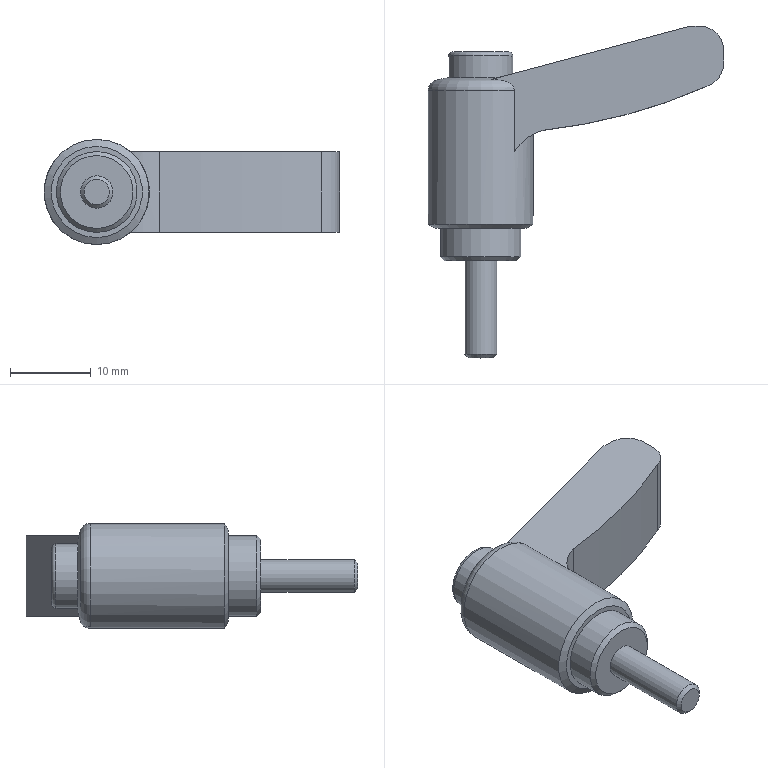Part | STEP file | CLDMC4-12-M | 2 solids | 40 faces | box 36.5 x 41 x 13 mm | volume 4938 mm3 | plane 23 | cylinder 10 | cone 4 | torus 2 | sphere 1 | commonest cylinder face diameters 6 x2 8 x2 10 x2 4 x1 12 x1 13 x1
STEP:
#1=CARTESIAN_POINT('',(-1.5,23.8,0.866));
#2=VERTEX_POINT('',#1);
#3=CARTESIAN_POINT('',(-0.75,23.8,1.299));
#4=VERTEX_POINT('',#3);
#5=CARTESIAN_POINT('',(-1.5,23.8,0.866));
#6=DIRECTION('',(0.866,0.,0.5));
#7=VECTOR('',#6,1000.);
#8=LINE('',#5,#7);
#9=EDGE_CURVE('',#2,#4,#8,.T.);
#10=ORIENTED_EDGE('',*,*,#9,.T.);
#11=CARTESIAN_POINT('',(-1.5,23.8,0.));
#12=VERTEX_POINT('',#11);
#13=CARTESIAN_POINT('',(0.,23.8,0.));
#14=DIRECTION('',(0.,1.,0.));
#15=DIRECTION('',(0.,0.,1.));
#16=AXIS2_PLACEMENT_3D('',#13,#14,#15);
#17=CIRCLE('',#16,1.5);
#18=EDGE_CURVE('',#4,#12,#17,.F.);
#19=ORIENTED_EDGE('',*,*,#18,.T.);
#20=CARTESIAN_POINT('',(-1.5,23.8,-0.866));
#21=DIRECTION('',(0.,0.,1.));
#22=VECTOR('',#21,1000.);
#23=LINE('',#20,#22);
#24=EDGE_CURVE('',#12,#2,#23,.T.);
#25=ORIENTED_EDGE('',*,*,#24,.T.);
#26=EDGE_LOOP('',(#10,#19,#25));
#27=FACE_OUTER_BOUND('',#26,.T.);
#28=CARTESIAN_POINT('',(0.,23.8,0.));
#29=DIRECTION('',(0.,1.,0.));
#30=DIRECTION('',(0.,0.,1.));
#31=AXIS2_PLACEMENT_3D('',#28,#29,#30);
#32=PLANE('',#31);
#33=ADVANCED_FACE('',(#27),#32,.T.);
#34=CARTESIAN_POINT('',(-1.5,23.8,-0.866));
#35=VERTEX_POINT('',#34);
#36=CARTESIAN_POINT('',(-1.5,23.8,-0.866));
#37=DIRECTION('',(0.,0.,1.));
#38=VECTOR('',#37,1000.);
#39=LINE('',#36,#38);
#40=EDGE_CURVE('',#35,#12,#39,.T.);
#41=ORIENTED_EDGE('',*,*,#40,.T.);
#42=CARTESIAN_POINT('',(-0.75,23.8,-1.299));
#43=VERTEX_POINT('',#42);
#44=CARTESIAN_POINT('',(0.,23.8,0.));
#45=DIRECTION('',(0.,1.,0.));
#46=DIRECTION('',(0.,0.,1.));
#47=AXIS2_PLACEMENT_3D('',#44,#45,#46);
#48=CIRCLE('',#47,1.5);
#49=EDGE_CURVE('',#12,#43,#48,.F.);
#50=ORIENTED_EDGE('',*,*,#49,.T.);
#51=CARTESIAN_POINT('',(0.,23.8,-1.732));
#52=DIRECTION('',(-0.866,0.,0.5));
#53=VECTOR('',#52,1000.);
#54=LINE('',#51,#53);
#55=EDGE_CURVE('',#43,#35,#54,.T.);
#56=ORIENTED_EDGE('',*,*,#55,.T.);
#57=EDGE_LOOP('',(#41,#50,#56));
#58=FACE_OUTER_BOUND('',#57,.T.);
#59=CARTESIAN_POINT('',(0.,23.8,0.));
#60=DIRECTION('',(0.,1.,0.));
#61=DIRECTION('',(0.,0.,1.));
#62=AXIS2_PLACEMENT_3D('',#59,#60,#61);
#63=PLANE('',#62);
#64=ADVANCED_FACE('',(#58),#63,.T.);
#65=CARTESIAN_POINT('',(0.,23.8,-1.732));
#66=VERTEX_POINT('',#65);
#67=CARTESIAN_POINT('',(0.,23.8,-1.732));
#68=DIRECTION('',(-0.866,0.,0.5));
#69=VECTOR('',#68,1000.);
#70=LINE('',#67,#69);
#71=EDGE_CURVE('',#66,#43,#70,.T.);
#72=ORIENTED_EDGE('',*,*,#71,.T.);
#73=CARTESIAN_POINT('',(0.,23.8,-1.5));
#74=VERTEX_POINT('',#73);
#75=CARTESIAN_POINT('',(0.,23.8,0.));
#76=DIRECTION('',(0.,1.,0.));
#77=DIRECTION('',(0.,0.,1.));
#78=AXIS2_PLACEMENT_3D('',#75,#76,#77);
#79=CIRCLE('',#78,1.5);
#80=EDGE_CURVE('',#43,#74,#79,.F.);
#81=ORIENTED_EDGE('',*,*,#80,.T.);
#82=CARTESIAN_POINT('',(0.75,23.8,-1.299));
#83=VERTEX_POINT('',#82);
#84=CARTESIAN_POINT('',(0.,23.8,0.));
#85=DIRECTION('',(0.,1.,0.));
#86=DIRECTION('',(0.,0.,1.));
#87=AXIS2_PLACEMENT_3D('',#84,#85,#86);
#88=CIRCLE('',#87,1.5);
#89=EDGE_CURVE('',#74,#83,#88,.F.);
#90=ORIENTED_EDGE('',*,*,#89,.T.);
#91=CARTESIAN_POINT('',(1.5,23.8,-0.866));
#92=DIRECTION('',(-0.866,0.,-0.5));
#93=VECTOR('',#92,1000.);
#94=LINE('',#91,#93);
#95=EDGE_CURVE('',#83,#66,#94,.T.);
#96=ORIENTED_EDGE('',*,*,#95,.T.);
#97=EDGE_LOOP('',(#72,#81,#90,#96));
#98=FACE_OUTER_BOUND('',#97,.T.);
#99=CARTESIAN_POINT('',(0.,23.8,0.));
#100=DIRECTION('',(0.,1.,0.));
#101=DIRECTION('',(0.,0.,1.));
#102=AXIS2_PLACEMENT_3D('',#99,#100,#101);
#103=PLANE('',#102);
#104=ADVANCED_FACE('',(#98),#103,.T.);
#105=CARTESIAN_POINT('',(1.5,23.8,-0.866));
#106=VERTEX_POINT('',#105);
#107=CARTESIAN_POINT('',(1.5,23.8,-0.866));
#108=DIRECTION('',(-0.866,0.,-0.5));
#109=VECTOR('',#108,1000.);
#110=LINE('',#107,#109);
#111=EDGE_CURVE('',#106,#83,#110,.T.);
#112=ORIENTED_EDGE('',*,*,#111,.T.);
#113=CARTESIAN_POINT('',(1.5,23.8,0.));
#114=VERTEX_POINT('',#113);
#115=CARTESIAN_POINT('',(0.,23.8,0.));
#116=DIRECTION('',(0.,1.,0.));
#117=DIRECTION('',(0.,0.,1.));
#118=AXIS2_PLACEMENT_3D('',#115,#116,#117);
#119=CIRCLE('',#118,1.5);
#120=EDGE_CURVE('',#83,#114,#119,.F.);
#121=ORIENTED_EDGE('',*,*,#120,.T.);
#122=CARTESIAN_POINT('',(1.5,23.8,0.866));
#123=DIRECTION('',(0.,0.,-1.));
#124=VECTOR('',#123,1000.);
#125=LINE('',#122,#124);
#126=EDGE_CURVE('',#114,#106,#125,.T.);
#127=ORIENTED_EDGE('',*,*,#126,.T.);
#128=EDGE_LOOP('',(#112,#121,#127));
#129=FACE_OUTER_BOUND('',#128,.T.);
#130=CARTESIAN_POINT('',(0.,23.8,0.));
#131=DIRECTION('',(0.,1.,0.));
#132=DIRECTION('',(0.,0.,1.));
#133=AXIS2_PLACEMENT_3D('',#130,#131,#132);
#134=PLANE('',#133);
#135=ADVANCED_FACE('',(#129),#134,.T.);
#136=CARTESIAN_POINT('',(1.5,23.8,0.866));
#137=VERTEX_POINT('',#136);
#138=CARTESIAN_POINT('',(1.5,23.8,0.866));
#139=DIRECTION('',(0.,0.,-1.));
#140=VECTOR('',#139,1000.);
#141=LINE('',#138,#140);
#142=EDGE_CURVE('',#137,#114,#141,.T.);
#143=ORIENTED_EDGE('',*,*,#142,.T.);
#144=CARTESIAN_POINT('',(0.75,23.8,1.299));
#145=VERTEX_POINT('',#144);
#146=CARTESIAN_POINT('',(0.,23.8,0.));
#147=DIRECTION('',(0.,-1.,0.));
#148=DIRECTION('',(0.,0.,-1.));
#149=AXIS2_PLACEMENT_3D('',#146,#147,#148);
#150=CIRCLE('',#149,1.5);
#151=EDGE_CURVE('',#114,#145,#150,.T.);
#152=ORIENTED_EDGE('',*,*,#151,.T.);
#153=CARTESIAN_POINT('',(0.,23.8,1.732));
#154=DIRECTION('',(0.866,0.,-0.5));
#155=VECTOR('',#154,1000.);
#156=LINE('',#153,#155);
#157=EDGE_CURVE('',#145,#137,#156,.T.);
#158=ORIENTED_EDGE('',*,*,#157,.T.);
#159=EDGE_LOOP('',(#143,#152,#158));
#160=FACE_OUTER_BOUND('',#159,.T.);
#161=CARTESIAN_POINT('',(0.,23.8,0.));
#162=DIRECTION('',(0.,1.,0.));
#163=DIRECTION('',(0.,0.,1.));
#164=AXIS2_PLACEMENT_3D('',#161,#162,#163);
#165=PLANE('',#164);
#166=ADVANCED_FACE('',(#160),#165,.T.);
#167=CARTESIAN_POINT('',(0.,25.8,-3.5));
#168=VERTEX_POINT('',#167);
#169=CARTESIAN_POINT('',(0.,25.8,3.5));
#170=VERTEX_POINT('',#169);
#171=CARTESIAN_POINT('',(0.,25.8,0.));
#172=DIRECTION('',(0.,-1.,0.));
#173=DIRECTION('',(0.,0.,-1.));
#174=AXIS2_PLACEMENT_3D('',#171,#172,#173);
#175=CIRCLE('',#174,3.5);
#176=EDGE_CURVE('',#168,#170,#175,.T.);
#177=ORIENTED_EDGE('',*,*,#176,.F.);
#178=CARTESIAN_POINT('',(0.,25.8,0.));
#179=DIRECTION('',(0.,-1.,0.));
#180=DIRECTION('',(0.,0.,-1.));
#181=AXIS2_PLACEMENT_3D('',#178,#179,#180);
#182=CIRCLE('',#181,3.5);
#183=EDGE_CURVE('',#170,#168,#182,.T.);
#184=ORIENTED_EDGE('',*,*,#183,.F.);
#185=EDGE_LOOP('',(#177,#184));
#186=FACE_OUTER_BOUND('',#185,.T.);
#187=CARTESIAN_POINT('',(-1.5,25.8,-0.866));
#188=VERTEX_POINT('',#187);
#189=CARTESIAN_POINT('',(-1.5,25.8,0.866));
#190=VERTEX_POINT('',#189);
#191=CARTESIAN_POINT('',(-1.5,25.8,0.));
#192=DIRECTION('',(0.,0.,1.));
#193=VECTOR('',#192,1000.);
#194=LINE('',#191,#193);
#195=EDGE_CURVE('',#188,#190,#194,.T.);
#196=ORIENTED_EDGE('',*,*,#195,.F.);
#197=CARTESIAN_POINT('',(0.,25.8,-1.732));
#198=VERTEX_POINT('',#197);
#199=CARTESIAN_POINT('',(-0.75,25.8,-1.299));
#200=DIRECTION('',(-0.866,0.,0.5));
#201=VECTOR('',#200,1000.);
#202=LINE('',#199,#201);
#203=EDGE_CURVE('',#198,#188,#202,.T.);
#204=ORIENTED_EDGE('',*,*,#203,.F.);
#205=CARTESIAN_POINT('',(1.5,25.8,-0.866));
#206=VERTEX_POINT('',#205);
#207=CARTESIAN_POINT('',(0.75,25.8,-1.299));
#208=DIRECTION('',(-0.866,0.,-0.5));
#209=VECTOR('',#208,1000.);
#210=LINE('',#207,#209);
#211=EDGE_CURVE('',#206,#198,#210,.T.);
#212=ORIENTED_EDGE('',*,*,#211,.F.);
#213=CARTESIAN_POINT('',(1.5,25.8,0.866));
#214=VERTEX_POINT('',#213);
#215=CARTESIAN_POINT('',(1.5,25.8,0.));
#216=DIRECTION('',(0.,0.,-1.));
#217=VECTOR('',#216,1000.);
#218=LINE('',#215,#217);
#219=EDGE_CURVE('',#214,#206,#218,.T.);
#220=ORIENTED_EDGE('',*,*,#219,.F.);
#221=CARTESIAN_POINT('',(0.,25.8,1.732));
#222=VERTEX_POINT('',#221);
#223=CARTESIAN_POINT('',(0.75,25.8,1.299));
#224=DIRECTION('',(0.866,0.,-0.5));
#225=VECTOR('',#224,1000.);
#226=LINE('',#223,#225);
#227=EDGE_CURVE('',#222,#214,#226,.T.);
#228=ORIENTED_EDGE('',*,*,#227,.F.);
#229=CARTESIAN_POINT('',(-0.75,25.8,1.299));
#230=DIRECTION('',(0.866,0.,0.5));
#231=VECTOR('',#230,1000.);
#232=LINE('',#229,#231);
#233=EDGE_CURVE('',#190,#222,#232,.T.);
#234=ORIENTED_EDGE('',*,*,#233,.F.);
#235=EDGE_LOOP('',(#196,#204,#212,#220,#228,#234));
#236=FACE_BOUND('',#235,.T.);
#237=CARTESIAN_POINT('',(0.,25.8,0.));
#238=DIRECTION('',(0.,-1.,0.));
#239=DIRECTION('',(0.,0.,-1.));
#240=AXIS2_PLACEMENT_3D('',#237,#238,#239);
#241=PLANE('',#240);
#242=ADVANCED_FACE('',(#186,#236),#241,.F.);
#243=CARTESIAN_POINT('',(0.,25.3,-4.));
#244=VERTEX_POINT('',#243);
#245=CARTESIAN_POINT('',(0.,25.3,4.));
#246=VERTEX_POINT('',#245);
#247=CARTESIAN_POINT('',(0.,25.3,0.));
#248=DIRECTION('',(0.,-1.,0.));
#249=DIRECTION('',(0.,0.,-1.));
#250=AXIS2_PLACEMENT_3D('',#247,#248,#249);
#251=CIRCLE('',#250,4.);
#252=EDGE_CURVE('',#244,#246,#251,.T.);
#253=ORIENTED_EDGE('',*,*,#252,.F.);
#254=CARTESIAN_POINT('',(0.,25.3,0.));
#255=DIRECTION('',(0.,-1.,0.));
#256=DIRECTION('',(0.,0.,-1.));
#257=AXIS2_PLACEMENT_3D('',#254,#255,#256);
#258=CIRCLE('',#257,4.);
#259=EDGE_CURVE('',#246,#244,#258,.T.);
#260=ORIENTED_EDGE('',*,*,#259,.F.);
#261=CARTESIAN_POINT('',(0.,25.3,3.5));
#262=DIRECTION('',(-1.,0.,0.));
#263=DIRECTION('',(0.,0.,1.));
#264=AXIS2_PLACEMENT_3D('',#261,#262,#263);
#265=CIRCLE('',#264,0.5);
#266=EDGE_CURVE('',#246,#170,#265,.T.);
#267=ORIENTED_EDGE('',*,*,#266,.T.);
#268=ORIENTED_EDGE('',*,*,#183,.T.);
#269=ORIENTED_EDGE('',*,*,#176,.T.);
#270=ORIENTED_EDGE('',*,*,#266,.F.);
#271=EDGE_LOOP('',(#253,#260,#267,#268,#269,#270));
#272=FACE_OUTER_BOUND('',#271,.T.);
#273=CARTESIAN_POINT('',(0.,25.3,0.));
#274=DIRECTION('',(0.,-1.,0.));
#275=DIRECTION('',(0.,0.,-1.));
#276=AXIS2_PLACEMENT_3D('',#273,#274,#275);
#277=TOROIDAL_SURFACE('',#276,3.5,0.5);
#278=ADVANCED_FACE('',(#272),#277,.T.);
#279=CARTESIAN_POINT('',(0.,12.9,-4.));
#280=VERTEX_POINT('',#279);
#281=CARTESIAN_POINT('',(0.,12.9,4.));
#282=VERTEX_POINT('',#281);
#283=CARTESIAN_POINT('',(0.,12.9,0.));
#284=DIRECTION('',(0.,-1.,0.));
#285=DIRECTION('',(0.,0.,-1.));
#286=AXIS2_PLACEMENT_3D('',#283,#284,#285);
#287=CIRCLE('',#286,4.);
#288=EDGE_CURVE('',#280,#282,#287,.T.);
#289=ORIENTED_EDGE('',*,*,#288,.F.);
#290=CARTESIAN_POINT('',(0.,12.9,0.));
#291=DIRECTION('',(0.,-1.,0.));
#292=DIRECTION('',(0.,0.,-1.));
#293=AXIS2_PLACEMENT_3D('',#290,#291,#292);
#294=CIRCLE('',#293,4.);
#295=EDGE_CURVE('',#282,#280,#294,.T.);
#296=ORIENTED_EDGE('',*,*,#295,.F.);
#297=CARTESIAN_POINT('',(0.,-12.,4.));
#298=DIRECTION('',(0.,1.,0.));
#299=VECTOR('',#298,4.);
#300=LINE('',#297,#299);
#301=EDGE_CURVE('',#282,#246,#300,.T.);
#302=ORIENTED_EDGE('',*,*,#301,.T.);
#303=ORIENTED_EDGE('',*,*,#259,.T.);
#304=ORIENTED_EDGE('',*,*,#252,.T.);
#305=ORIENTED_EDGE('',*,*,#301,.F.);
#306=EDGE_LOOP('',(#289,#296,#302,#303,#304,#305));
#307=FACE_OUTER_BOUND('',#306,.T.);
#308=CARTESIAN_POINT('',(0.,-12.,0.));
#309=DIRECTION('',(0.,-1.,0.));
#310=DIRECTION('',(0.,0.,-1.));
#311=AXIS2_PLACEMENT_3D('',#308,#309,#310);
#312=CYLINDRICAL_SURFACE('',#311,4.);
#313=ADVANCED_FACE('',(#307),#312,.T.);
#314=CARTESIAN_POINT('',(0.,12.9,-5.));
#315=VERTEX_POINT('',#314);
#316=CARTESIAN_POINT('',(0.,12.9,5.));
#317=VERTEX_POINT('',#316);
#318=CARTESIAN_POINT('',(0.,12.9,0.));
#319=DIRECTION('',(0.,-1.,0.));
#320=DIRECTION('',(0.,0.,-1.));
#321=AXIS2_PLACEMENT_3D('',#318,#319,#320);
#322=CIRCLE('',#321,5.);
#323=EDGE_CURVE('',#315,#317,#322,.T.);
#324=ORIENTED_EDGE('',*,*,#323,.F.);
#325=CARTESIAN_POINT('',(0.,12.9,0.));
#326=DIRECTION('',(0.,-1.,0.));
#327=DIRECTION('',(0.,0.,-1.));
#328=AXIS2_PLACEMENT_3D('',#325,#326,#327);
#329=CIRCLE('',#328,5.);
#330=EDGE_CURVE('',#317,#315,#329,.T.);
#331=ORIENTED_EDGE('',*,*,#330,.F.);
#332=EDGE_LOOP('',(#324,#331));
#333=FACE_OUTER_BOUND('',#332,.T.);
#334=ORIENTED_EDGE('',*,*,#288,.T.);
#335=ORIENTED_EDGE('',*,*,#295,.T.);
#336=EDGE_LOOP('',(#334,#335));
#337=FACE_BOUND('',#336,.T.);
#338=CARTESIAN_POINT('',(4.,12.9,0.));
#339=DIRECTION('',(0.,-1.,0.));
#340=DIRECTION('',(0.,0.,-1.));
#341=AXIS2_PLACEMENT_3D('',#338,#339,#340);
#342=PLANE('',#341);
#343=ADVANCED_FACE('',(#333,#337),#342,.F.);
#344=CARTESIAN_POINT('',(0.,0.5,-5.));
#345=VERTEX_POINT('',#344);
#346=CARTESIAN_POINT('',(0.,0.5,5.));
#347=VERTEX_POINT('',#346);
#348=CARTESIAN_POINT('',(0.,0.5,0.));
#349=DIRECTION('',(0.,-1.,0.));
#350=DIRECTION('',(0.,0.,-1.));
#351=AXIS2_PLACEMENT_3D('',#348,#349,#350);
#352=CIRCLE('',#351,5.);
#353=EDGE_CURVE('',#345,#347,#352,.T.);
#354=ORIENTED_EDGE('',*,*,#353,.F.);
#355=CARTESIAN_POINT('',(0.,0.5,0.));
#356=DIRECTION('',(0.,-1.,0.));
#357=DIRECTION('',(0.,0.,-1.));
#358=AXIS2_PLACEMENT_3D('',#355,#356,#357);
#359=CIRCLE('',#358,5.);
#360=EDGE_CURVE('',#347,#345,#359,.T.);
#361=ORIENTED_EDGE('',*,*,#360,.F.);
#362=CARTESIAN_POINT('',(0.,-12.,5.));
#363=DIRECTION('',(0.,1.,0.));
#364=VECTOR('',#363,5.);
#365=LINE('',#362,#364);
#366=EDGE_CURVE('',#347,#317,#365,.T.);
#367=ORIENTED_EDGE('',*,*,#366,.T.);
#368=ORIENTED_EDGE('',*,*,#330,.T.);
#369=ORIENTED_EDGE('',*,*,#323,.T.);
#370=ORIENTED_EDGE('',*,*,#366,.F.);
#371=EDGE_LOOP('',(#354,#361,#367,#368,#369,#370));
#372=FACE_OUTER_BOUND('',#371,.T.);
#373=CARTESIAN_POINT('',(0.,-12.,0.));
#374=DIRECTION('',(0.,-1.,0.));
#375=DIRECTION('',(0.,0.,-1.));
#376=AXIS2_PLACEMENT_3D('',#373,#374,#375);
#377=CYLINDRICAL_SURFACE('',#376,5.);
#378=ADVANCED_FACE('',(#372),#377,.T.);
#379=ORIENTED_EDGE('',*,*,#353,.T.);
#380=ORIENTED_EDGE('',*,*,#360,.T.);
#381=CARTESIAN_POINT('',(0.,0.,-4.5));
#382=VERTEX_POINT('',#381);
#383=CARTESIAN_POINT('',(0.,0.5,-5.));
#384=DIRECTION('',(0.,-0.7071,0.7071));
#385=VECTOR('',#384,5.);
#386=LINE('',#383,#385);
#387=EDGE_CURVE('',#345,#382,#386,.T.);
#388=ORIENTED_EDGE('',*,*,#387,.T.);
#389=CARTESIAN_POINT('',(0.,0.,0.));
#390=DIRECTION('',(0.,-1.,0.));
#391=DIRECTION('',(0.,0.,-1.));
#392=AXIS2_PLACEMENT_3D('',#389,#390,#391);
#393=CIRCLE('',#392,4.5);
#394=EDGE_CURVE('',#382,#382,#393,.T.);
#395=ORIENTED_EDGE('',*,*,#394,.F.);
#396=ORIENTED_EDGE('',*,*,#387,.F.);
#397=EDGE_LOOP('',(#379,#380,#388,#395,#396));
#398=FACE_OUTER_BOUND('',#397,.T.);
#399=CARTESIAN_POINT('',(0.,0.5,0.));
#400=DIRECTION('',(0.,1.,0.));
#401=DIRECTION('',(0.,0.,1.));
#402=AXIS2_PLACEMENT_3D('',#399,#400,#401);
#403=CONICAL_SURFACE('',#402,5.,0.7854);
#404=ADVANCED_FACE('',(#398),#403,.T.);
#405=ORIENTED_EDGE('',*,*,#394,.T.);
#406=EDGE_LOOP('',(#405));
#407=FACE_OUTER_BOUND('',#406,.T.);
#408=CARTESIAN_POINT('',(0.,0.,-2.));
#409=VERTEX_POINT('',#408);
#410=CARTESIAN_POINT('',(0.,0.,2.));
#411=VERTEX_POINT('',#410);
#412=CARTESIAN_POINT('',(0.,0.,0.));
#413=DIRECTION('',(0.,-1.,0.));
#414=DIRECTION('',(0.,0.,-1.));
#415=AXIS2_PLACEMENT_3D('',#412,#413,#414);
#416=CIRCLE('',#415,2.);
#417=EDGE_CURVE('',#409,#411,#416,.T.);
#418=ORIENTED_EDGE('',*,*,#417,.F.);
#419=CARTESIAN_POINT('',(0.,0.,0.));
#420=DIRECTION('',(0.,-1.,0.));
#421=DIRECTION('',(0.,0.,-1.));
#422=AXIS2_PLACEMENT_3D('',#419,#420,#421);
#423=CIRCLE('',#422,2.);
#424=EDGE_CURVE('',#411,#409,#423,.T.);
#425=ORIENTED_EDGE('',*,*,#424,.F.);
#426=EDGE_LOOP('',(#418,#425));
#427=FACE_BOUND('',#426,.T.);
#428=CARTESIAN_POINT('',(4.5,0.,0.));
#429=DIRECTION('',(0.,1.,0.));
#430=DIRECTION('',(0.,0.,1.));
#431=AXIS2_PLACEMENT_3D('',#428,#429,#430);
#432=PLANE('',#431);
#433=ADVANCED_FACE('',(#407,#427),#432,.F.);
#434=CARTESIAN_POINT('',(0.,-11.57,-2.));
#435=VERTEX_POINT('',#434);
#436=CARTESIAN_POINT('',(0.,-11.57,2.));
#437=VERTEX_POINT('',#436);
#438=CARTESIAN_POINT('',(0.,-11.57,0.));
#439=DIRECTION('',(0.,-1.,0.));
#440=DIRECTION('',(0.,0.,-1.));
#441=AXIS2_PLACEMENT_3D('',#438,#439,#440);
#442=CIRCLE('',#441,2.);
#443=EDGE_CURVE('',#435,#437,#442,.T.);
#444=ORIENTED_EDGE('',*,*,#443,.F.);
#445=CARTESIAN_POINT('',(0.,-11.57,0.));
#446=DIRECTION('',(0.,-1.,0.));
#447=DIRECTION('',(0.,0.,-1.));
#448=AXIS2_PLACEMENT_3D('',#445,#446,#447);
#449=CIRCLE('',#448,2.);
#450=EDGE_CURVE('',#437,#435,#449,.T.);
#451=ORIENTED_EDGE('',*,*,#450,.F.);
#452=CARTESIAN_POINT('',(0.,-12.,2.));
#453=DIRECTION('',(0.,1.,0.));
#454=VECTOR('',#453,2.);
#455=LINE('',#452,#454);
#456=EDGE_CURVE('',#437,#411,#455,.T.);
#457=ORIENTED_EDGE('',*,*,#456,.T.);
#458=ORIENTED_EDGE('',*,*,#424,.T.);
#459=ORIENTED_EDGE('',*,*,#417,.T.);
#460=ORIENTED_EDGE('',*,*,#456,.F.);
#461=EDGE_LOOP('',(#444,#451,#457,#458,#459,#460));
#462=FACE_OUTER_BOUND('',#461,.T.);
#463=CARTESIAN_POINT('',(0.,-12.,0.));
#464=DIRECTION('',(0.,-1.,0.));
#465=DIRECTION('',(0.,0.,-1.));
#466=AXIS2_PLACEMENT_3D('',#463,#464,#465);
#467=CYLINDRICAL_SURFACE('',#466,2.);
#468=ADVANCED_FACE('',(#462),#467,.T.);
#469=ORIENTED_EDGE('',*,*,#443,.T.);
#470=ORIENTED_EDGE('',*,*,#450,.T.);
#471=CARTESIAN_POINT('',(0.,-12.,-1.571));
#472=VERTEX_POINT('',#471);
#473=CARTESIAN_POINT('',(0.,-11.57,-2.));
#474=DIRECTION('',(0.,-0.7071,0.7071));
#475=VECTOR('',#474,2.);
#476=LINE('',#473,#475);
#477=EDGE_CURVE('',#435,#472,#476,.T.);
#478=ORIENTED_EDGE('',*,*,#477,.T.);
#479=CARTESIAN_POINT('',(0.,-12.,0.));
#480=DIRECTION('',(0.,-1.,0.));
#481=DIRECTION('',(0.,0.,-1.));
#482=AXIS2_PLACEMENT_3D('',#479,#480,#481);
#483=CIRCLE('',#482,1.571);
#484=EDGE_CURVE('',#472,#472,#483,.T.);
#485=ORIENTED_EDGE('',*,*,#484,.F.);
#486=ORIENTED_EDGE('',*,*,#477,.F.);
#487=EDGE_LOOP('',(#469,#470,#478,#485,#486));
#488=FACE_OUTER_BOUND('',#487,.T.);
#489=CARTESIAN_POINT('',(0.,-11.57,0.));
#490=DIRECTION('',(0.,1.,0.));
#491=DIRECTION('',(0.,0.,1.));
#492=AXIS2_PLACEMENT_3D('',#489,#490,#491);
#493=CONICAL_SURFACE('',#492,2.,0.7854);
#494=ADVANCED_FACE('',(#488),#493,.T.);
#495=ORIENTED_EDGE('',*,*,#484,.T.);
#496=EDGE_LOOP('',(#495));
#497=FACE_OUTER_BOUND('',#496,.T.);
#498=CARTESIAN_POINT('',(1.571,-12.,0.));
#499=DIRECTION('',(0.,1.,0.));
#500=DIRECTION('',(0.,0.,1.));
#501=AXIS2_PLACEMENT_3D('',#498,#499,#500);
#502=PLANE('',#501);
#503=ADVANCED_FACE('',(#497),#502,.F.);
#504=ORIENTED_EDGE('',*,*,#195,.T.);
#505=CARTESIAN_POINT('',(-1.5,27.8,0.866));
#506=DIRECTION('',(0.,-1.,0.));
#507=VECTOR('',#506,1000.);
#508=LINE('',#505,#507);
#509=EDGE_CURVE('',#190,#2,#508,.T.);
#510=ORIENTED_EDGE('',*,*,#509,.T.);
#511=ORIENTED_EDGE('',*,*,#24,.F.);
#512=ORIENTED_EDGE('',*,*,#40,.F.);
#513=CARTESIAN_POINT('',(-1.5,27.8,-0.866));
#514=DIRECTION('',(0.,-1.,0.));
#515=VECTOR('',#514,1000.);
#516=LINE('',#513,#515);
#517=EDGE_CURVE('',#188,#35,#516,.T.);
#518=ORIENTED_EDGE('',*,*,#517,.F.);
#519=EDGE_LOOP('',(#504,#510,#511,#512,#518));
#520=FACE_OUTER_BOUND('',#519,.T.);
#521=CARTESIAN_POINT('',(-1.5,27.8,-0.866));
#522=DIRECTION('',(1.,0.,0.));
#523=DIRECTION('',(0.,0.,-1.));
#524=AXIS2_PLACEMENT_3D('',#521,#522,#523);
#525=PLANE('',#524);
#526=ADVANCED_FACE('',(#520),#525,.T.);
#527=ORIENTED_EDGE('',*,*,#233,.T.);
#528=CARTESIAN_POINT('',(0.,23.8,1.732));
#529=VERTEX_POINT('',#528);
#530=CARTESIAN_POINT('',(0.,27.8,1.732));
#531=DIRECTION('',(0.,-1.,0.));
#532=VECTOR('',#531,1000.);
#533=LINE('',#530,#532);
#534=EDGE_CURVE('',#222,#529,#533,.T.);
#535=ORIENTED_EDGE('',*,*,#534,.T.);
#536=CARTESIAN_POINT('',(-1.5,23.8,0.866));
#537=DIRECTION('',(0.866,0.,0.5));
#538=VECTOR('',#537,1000.);
#539=LINE('',#536,#538);
#540=EDGE_CURVE('',#4,#529,#539,.T.);
#541=ORIENTED_EDGE('',*,*,#540,.F.);
#542=ORIENTED_EDGE('',*,*,#9,.F.);
#543=ORIENTED_EDGE('',*,*,#509,.F.);
#544=EDGE_LOOP('',(#527,#535,#541,#542,#543));
#545=FACE_OUTER_BOUND('',#544,.T.);
#546=CARTESIAN_POINT('',(-1.5,27.8,0.866));
#547=DIRECTION('',(0.5,0.,-0.866));
#548=DIRECTION('',(-0.866,0.,-0.5));
#549=AXIS2_PLACEMENT_3D('',#546,#547,#548);
#550=PLANE('',#549);
#551=ADVANCED_FACE('',(#545),#550,.T.);
#552=ORIENTED_EDGE('',*,*,#227,.T.);
#553=CARTESIAN_POINT('',(1.5,27.8,0.866));
#554=DIRECTION('',(0.,-1.,0.));
#555=VECTOR('',#554,1000.);
#556=LINE('',#553,#555);
#557=EDGE_CURVE('',#214,#137,#556,.T.);
#558=ORIENTED_EDGE('',*,*,#557,.T.);
#559=ORIENTED_EDGE('',*,*,#157,.F.);
#560=CARTESIAN_POINT('',(0.,23.8,1.732));
#561=DIRECTION('',(0.866,0.,-0.5));
#562=VECTOR('',#561,1000.);
#563=LINE('',#560,#562);
#564=EDGE_CURVE('',#529,#145,#563,.T.);
#565=ORIENTED_EDGE('',*,*,#564,.F.);
#566=ORIENTED_EDGE('',*,*,#534,.F.);
#567=EDGE_LOOP('',(#552,#558,#559,#565,#566));
#568=FACE_OUTER_BOUND('',#567,.T.);
#569=CARTESIAN_POINT('',(0.,27.8,1.732));
#570=DIRECTION('',(-0.5,0.,-0.866));
#571=DIRECTION('',(-0.866,0.,0.5));
#572=AXIS2_PLACEMENT_3D('',#569,#570,#571);
#573=PLANE('',#572);
#574=ADVANCED_FACE('',(#568),#573,.T.);
#575=ORIENTED_EDGE('',*,*,#557,.F.);
#576=ORIENTED_EDGE('',*,*,#219,.T.);
#577=CARTESIAN_POINT('',(1.5,27.8,-0.866));
#578=DIRECTION('',(0.,-1.,0.));
#579=VECTOR('',#578,1000.);
#580=LINE('',#577,#579);
#581=EDGE_CURVE('',#206,#106,#580,.T.);
#582=ORIENTED_EDGE('',*,*,#581,.T.);
#583=ORIENTED_EDGE('',*,*,#126,.F.);
#584=ORIENTED_EDGE('',*,*,#142,.F.);
#585=EDGE_LOOP('',(#575,#576,#582,#583,#584));
#586=FACE_OUTER_BOUND('',#585,.T.);
#587=CARTESIAN_POINT('',(1.5,27.8,0.866));
#588=DIRECTION('',(-1.,0.,0.));
#589=DIRECTION('',(0.,0.,1.));
#590=AXIS2_PLACEMENT_3D('',#587,#588,#589);
#591=PLANE('',#590);
#592=ADVANCED_FACE('',(#586),#591,.T.);
#593=ORIENTED_EDGE('',*,*,#211,.T.);
#594=CARTESIAN_POINT('',(0.,27.8,-1.732));
#595=DIRECTION('',(0.,-1.,0.));
#596=VECTOR('',#595,1000.);
#597=LINE('',#594,#596);
#598=EDGE_CURVE('',#198,#66,#597,.T.);
#599=ORIENTED_EDGE('',*,*,#598,.T.);
#600=ORIENTED_EDGE('',*,*,#95,.F.);
#601=ORIENTED_EDGE('',*,*,#111,.F.);
#602=ORIENTED_EDGE('',*,*,#581,.F.);
#603=EDGE_LOOP('',(#593,#599,#600,#601,#602));
#604=FACE_OUTER_BOUND('',#603,.T.);
#605=CARTESIAN_POINT('',(1.5,27.8,-0.866));
#606=DIRECTION('',(-0.5,0.,0.866));
#607=DIRECTION('',(0.866,0.,0.5));
#608=AXIS2_PLACEMENT_3D('',#605,#606,#607);
#609=PLANE('',#608);
#610=ADVANCED_FACE('',(#604),#609,.T.);
#611=ORIENTED_EDGE('',*,*,#203,.T.);
#612=ORIENTED_EDGE('',*,*,#517,.T.);
#613=ORIENTED_EDGE('',*,*,#55,.F.);
#614=ORIENTED_EDGE('',*,*,#71,.F.);
#615=ORIENTED_EDGE('',*,*,#598,.F.);
#616=EDGE_LOOP('',(#611,#612,#613,#614,#615));
#617=FACE_OUTER_BOUND('',#616,.T.);
#618=CARTESIAN_POINT('',(0.,27.8,-1.732));
#619=DIRECTION('',(0.5,0.,0.866));
#620=DIRECTION('',(0.866,0.,-0.5));
#621=AXIS2_PLACEMENT_3D('',#618,#619,#620);
#622=PLANE('',#621);
#623=ADVANCED_FACE('',(#617),#622,.T.);
#624=ORIENTED_EDGE('',*,*,#564,.T.);
#625=CARTESIAN_POINT('',(0.,23.8,0.));
#626=DIRECTION('',(0.,1.,0.));
#627=DIRECTION('',(0.,0.,1.));
#628=AXIS2_PLACEMENT_3D('',#625,#626,#627);
#629=CIRCLE('',#628,1.5);
#630=EDGE_CURVE('',#145,#4,#629,.F.);
#631=ORIENTED_EDGE('',*,*,#630,.T.);
#632=ORIENTED_EDGE('',*,*,#540,.T.);
#633=EDGE_LOOP('',(#624,#631,#632));
#634=FACE_OUTER_BOUND('',#633,.T.);
#635=CARTESIAN_POINT('',(0.,23.8,0.));
#636=DIRECTION('',(0.,1.,0.));
#637=DIRECTION('',(0.,0.,1.));
#638=AXIS2_PLACEMENT_3D('',#635,#636,#637);
#639=PLANE('',#638);
#640=ADVANCED_FACE('',(#634),#639,.T.);
#641=CARTESIAN_POINT('',(0.,22.934,0.));
#642=VERTEX_POINT('',#641);
#643=CARTESIAN_POINT('',(0.,23.8,-1.5));
#644=DIRECTION('',(0.,0.5,-0.866));
#645=VECTOR('',#644,1.5);
#646=LINE('',#643,#645);
#647=EDGE_CURVE('',#642,#74,#646,.T.);
#648=ORIENTED_EDGE('',*,*,#647,.T.);
#649=ORIENTED_EDGE('',*,*,#80,.F.);
#650=ORIENTED_EDGE('',*,*,#49,.F.);
#651=ORIENTED_EDGE('',*,*,#18,.F.);
#652=ORIENTED_EDGE('',*,*,#630,.F.);
#653=ORIENTED_EDGE('',*,*,#151,.F.);
#654=ORIENTED_EDGE('',*,*,#120,.F.);
#655=ORIENTED_EDGE('',*,*,#89,.F.);
#656=ORIENTED_EDGE('',*,*,#647,.F.);
#657=EDGE_LOOP('',(#648,#649,#650,#651,#652,#653,#654,#655,#656));
#658=FACE_OUTER_BOUND('',#657,.T.);
#659=CARTESIAN_POINT('',(0.,23.8,0.));
#660=DIRECTION('',(0.,1.,0.));
#661=DIRECTION('',(0.,0.,1.));
#662=AXIS2_PLACEMENT_3D('',#659,#660,#661);
#663=CONICAL_SURFACE('',#662,1.5,1.047);
#664=ADVANCED_FACE('',(#658),#663,.F.);
#665=CLOSED_SHELL('',(#33,#64,#104,#135,#166,#242,#278,#313,#343,#378,#404,#433,#468,#494,#503,#526,#551,#574,#592,#610,#623,#640,#664));
#666=MANIFOLD_SOLID_BREP('',#665);
#667=CARTESIAN_POINT('',(1.3,22.4,5.));
#668=VERTEX_POINT('',#667);
#669=CARTESIAN_POINT('',(2.161,22.63,3.366));
#670=VERTEX_POINT('',#669);
#671=CARTESIAN_POINT('',(-5.674,20.531,0.));
#672=DIRECTION('',(0.2588,-0.9659,0.));
#673=DIRECTION('',(0.9659,0.2588,0.));
#674=AXIS2_PLACEMENT_3D('',#671,#672,#673);
#675=CIRCLE('',#674,8.782);
#676=EDGE_CURVE('',#668,#670,#675,.F.);
#677=ORIENTED_EDGE('',*,*,#676,.T.);
#678=CARTESIAN_POINT('',(0.,22.63,4.));
#679=VERTEX_POINT('',#678);
#680=CARTESIAN_POINT('',(0.,22.63,0.));
#681=DIRECTION('',(0.,-1.,0.));
#682=DIRECTION('',(0.,0.,-1.));
#683=AXIS2_PLACEMENT_3D('',#680,#681,#682);
#684=CIRCLE('',#683,4.);
#685=EDGE_CURVE('',#670,#679,#684,.T.);
#686=ORIENTED_EDGE('',*,*,#685,.T.);
#687=CARTESIAN_POINT('',(2.161,22.63,-3.366));
#688=VERTEX_POINT('',#687);
#689=CARTESIAN_POINT('',(0.,22.63,0.));
#690=DIRECTION('',(0.,-1.,0.));
#691=DIRECTION('',(0.,0.,-1.));
#692=AXIS2_PLACEMENT_3D('',#689,#690,#691);
#693=CIRCLE('',#692,4.);
#694=EDGE_CURVE('',#679,#688,#693,.T.);
#695=ORIENTED_EDGE('',*,*,#694,.T.);
#696=CARTESIAN_POINT('',(1.3,22.4,-5.));
#697=VERTEX_POINT('',#696);
#698=CARTESIAN_POINT('',(-5.674,20.531,0.));
#699=DIRECTION('',(0.2588,-0.9659,0.));
#700=DIRECTION('',(0.9659,0.2588,0.));
#701=AXIS2_PLACEMENT_3D('',#698,#699,#700);
#702=CIRCLE('',#701,8.782);
#703=EDGE_CURVE('',#688,#697,#702,.F.);
#704=ORIENTED_EDGE('',*,*,#703,.T.);
#705=CARTESIAN_POINT('',(2.298,22.322,-5.));
#706=VERTEX_POINT('',#705);
#707=CARTESIAN_POINT('',(0.,-0.6437,-5.));
#708=DIRECTION('',(0.,0.,1.));
#709=DIRECTION('',(1.,0.,0.));
#710=AXIS2_PLACEMENT_3D('',#707,#708,#709);
#711=CIRCLE('',#710,23.08);
#712=EDGE_CURVE('',#697,#706,#711,.F.);
#713=ORIENTED_EDGE('',*,*,#712,.T.);
#714=CARTESIAN_POINT('',(2.298,22.322,5.));
#715=VERTEX_POINT('',#714);
#716=CARTESIAN_POINT('',(0.,22.322,0.));
#717=DIRECTION('',(0.,-1.,0.));
#718=DIRECTION('',(0.,0.,-1.));
#719=AXIS2_PLACEMENT_3D('',#716,#717,#718);
#720=CIRCLE('',#719,5.503);
#721=EDGE_CURVE('',#715,#706,#720,.T.);
#722=ORIENTED_EDGE('',*,*,#721,.F.);
#723=CARTESIAN_POINT('',(0.,-0.6437,5.));
#724=DIRECTION('',(0.,0.,1.));
#725=DIRECTION('',(1.,0.,0.));
#726=AXIS2_PLACEMENT_3D('',#723,#724,#725);
#727=CIRCLE('',#726,23.08);
#728=EDGE_CURVE('',#668,#715,#727,.F.);
#729=ORIENTED_EDGE('',*,*,#728,.F.);
#730=EDGE_LOOP('',(#677,#686,#695,#704,#713,#722,#729));
#731=FACE_OUTER_BOUND('',#730,.T.);
#732=CARTESIAN_POINT('',(0.,-0.6437,0.));
#733=DIRECTION('',(0.,-1.,0.));
#734=DIRECTION('',(-1.,0.,0.));
#735=AXIS2_PLACEMENT_3D('',#732,#733,#734);
#736=SPHERICAL_SURFACE('',#735,23.615);
#737=ADVANCED_FACE('',(#731),#736,.T.);
#738=CARTESIAN_POINT('',(4.153,21.057,5.));
#739=VERTEX_POINT('',#738);
#740=CARTESIAN_POINT('',(2.298,22.322,5.));
#741=CARTESIAN_POINT('',(2.567,22.295,5.));
#742=CARTESIAN_POINT('',(2.832,22.247,5.));
#743=CARTESIAN_POINT('',(3.292,22.104,5.));
#744=CARTESIAN_POINT('',(3.546,21.986,5.));
#745=CARTESIAN_POINT('',(3.856,21.74,5.));
#746=CARTESIAN_POINT('',(3.984,21.595,5.));
#747=CARTESIAN_POINT('',(4.115,21.336,5.));
#748=CARTESIAN_POINT('',(4.153,21.186,5.));
#749=CARTESIAN_POINT('',(4.153,21.057,5.));
#750=B_SPLINE_CURVE_WITH_KNOTS('',3,(#740,#741,#742,#743,#744,#745,#746,#747,#748,#749),.UNSPECIFIED.,.F.,.F.,(4,2,2,2,4),(0.2157,0.29,0.3601,0.4085,0.4472),.UNSPECIFIED.);
#751=EDGE_CURVE('',#715,#739,#750,.T.);
#752=ORIENTED_EDGE('',*,*,#751,.F.);
#753=ORIENTED_EDGE('',*,*,#721,.T.);
#754=CARTESIAN_POINT('',(4.153,21.057,-5.));
#755=VERTEX_POINT('',#754);
#756=CARTESIAN_POINT('',(2.298,22.322,-5.));
#757=CARTESIAN_POINT('',(2.567,22.295,-5.));
#758=CARTESIAN_POINT('',(2.832,22.247,-5.));
#759=CARTESIAN_POINT('',(3.292,22.104,-5.));
#760=CARTESIAN_POINT('',(3.546,21.986,-5.));
#761=CARTESIAN_POINT('',(3.856,21.74,-5.));
#762=CARTESIAN_POINT('',(3.984,21.595,-5.));
#763=CARTESIAN_POINT('',(4.115,21.336,-5.));
#764=CARTESIAN_POINT('',(4.153,21.186,-5.));
#765=CARTESIAN_POINT('',(4.153,21.057,-5.));
#766=B_SPLINE_CURVE_WITH_KNOTS('',3,(#756,#757,#758,#759,#760,#761,#762,#763,#764,#765),.UNSPECIFIED.,.F.,.F.,(4,2,2,2,4),(0.2157,0.29,0.3601,0.4085,0.4472),.UNSPECIFIED.);
#767=EDGE_CURVE('',#706,#755,#766,.T.);
#768=ORIENTED_EDGE('',*,*,#767,.T.);
#769=CARTESIAN_POINT('',(0.,21.057,6.5));
#770=VERTEX_POINT('',#769);
#771=CARTESIAN_POINT('',(0.,21.057,0.));
#772=DIRECTION('',(0.,-1.,0.));
#773=DIRECTION('',(0.,0.,-1.));
#774=AXIS2_PLACEMENT_3D('',#771,#772,#773);
#775=CIRCLE('',#774,6.5);
#776=EDGE_CURVE('',#770,#755,#775,.T.);
#777=ORIENTED_EDGE('',*,*,#776,.F.);
#778=CARTESIAN_POINT('',(0.,21.057,0.));
#779=DIRECTION('',(0.,-1.,0.));
#780=DIRECTION('',(0.,0.,-1.));
#781=AXIS2_PLACEMENT_3D('',#778,#779,#780);
#782=CIRCLE('',#781,6.5);
#783=EDGE_CURVE('',#739,#770,#782,.T.);
#784=ORIENTED_EDGE('',*,*,#783,.F.);
#785=EDGE_LOOP('',(#752,#753,#768,#777,#784));
#786=FACE_OUTER_BOUND('',#785,.T.);
#787=CARTESIAN_POINT('',(0.,21.057,0.));
#788=DIRECTION('',(0.,-1.,0.));
#789=DIRECTION('',(-1.,0.,0.));
#790=AXIS2_PLACEMENT_3D('',#787,#788,#789);
#791=TOROIDAL_SURFACE('',#790,5.2,1.3);
#792=ADVANCED_FACE('',(#786),#791,.T.);
#793=CARTESIAN_POINT('',(0.,4.5,-6.5));
#794=VERTEX_POINT('',#793);
#795=CARTESIAN_POINT('',(0.,4.5,6.5));
#796=VERTEX_POINT('',#795);
#797=CARTESIAN_POINT('',(0.,4.5,0.));
#798=DIRECTION('',(0.,-1.,0.));
#799=DIRECTION('',(0.,0.,-1.));
#800=AXIS2_PLACEMENT_3D('',#797,#798,#799);
#801=CIRCLE('',#800,6.5);
#802=EDGE_CURVE('',#794,#796,#801,.T.);
#803=ORIENTED_EDGE('',*,*,#802,.F.);
#804=CARTESIAN_POINT('',(0.,4.5,0.));
#805=DIRECTION('',(0.,-1.,0.));
#806=DIRECTION('',(0.,0.,-1.));
#807=AXIS2_PLACEMENT_3D('',#804,#805,#806);
#808=CIRCLE('',#807,6.5);
#809=EDGE_CURVE('',#796,#794,#808,.T.);
#810=ORIENTED_EDGE('',*,*,#809,.F.);
#811=CARTESIAN_POINT('',(0.,4.,6.5));
#812=DIRECTION('',(0.,1.,0.));
#813=VECTOR('',#812,6.5);
#814=LINE('',#811,#813);
#815=EDGE_CURVE('',#796,#770,#814,.T.);
#816=ORIENTED_EDGE('',*,*,#815,.T.);
#817=ORIENTED_EDGE('',*,*,#776,.T.);
#818=CARTESIAN_POINT('',(4.153,13.493,-5.));
#819=VERTEX_POINT('',#818);
#820=CARTESIAN_POINT('',(4.153,4.,-5.));
#821=DIRECTION('',(0.,-1.,0.));
#822=VECTOR('',#821,1000.);
#823=LINE('',#820,#822);
#824=EDGE_CURVE('',#819,#755,#823,.F.);
#825=ORIENTED_EDGE('',*,*,#824,.F.);
#826=CARTESIAN_POINT('',(4.153,13.493,5.));
#827=VERTEX_POINT('',#826);
#828=CARTESIAN_POINT('',(4.153,13.493,-5.));
#829=CARTESIAN_POINT('',(4.292,13.716,-4.885));
#830=CARTESIAN_POINT('',(4.44,13.921,-4.752));
#831=CARTESIAN_POINT('',(4.752,14.306,-4.441));
#832=CARTESIAN_POINT('',(4.935,14.503,-4.24));
#833=CARTESIAN_POINT('',(5.291,14.842,-3.786));
#834=CARTESIAN_POINT('',(5.463,14.984,-3.534));
#835=CARTESIAN_POINT('',(5.871,15.295,-2.838));
#836=CARTESIAN_POINT('',(6.108,15.441,-2.3));
#837=CARTESIAN_POINT('',(6.423,15.622,-1.159));
#838=CARTESIAN_POINT('',(6.5,15.659,-0.5571));
#839=CARTESIAN_POINT('',(6.5,15.659,0.5571));
#840=CARTESIAN_POINT('',(6.423,15.622,1.159));
#841=CARTESIAN_POINT('',(6.108,15.441,2.3));
#842=CARTESIAN_POINT('',(5.871,15.295,2.838));
#843=CARTESIAN_POINT('',(5.463,14.984,3.534));
#844=CARTESIAN_POINT('',(5.291,14.842,3.786));
#845=CARTESIAN_POINT('',(4.935,14.503,4.24));
#846=CARTESIAN_POINT('',(4.752,14.306,4.441));
#847=CARTESIAN_POINT('',(4.44,13.921,4.752));
#848=CARTESIAN_POINT('',(4.292,13.716,4.885));
#849=CARTESIAN_POINT('',(4.153,13.493,5.));
#850=B_SPLINE_CURVE_WITH_KNOTS('',3,(#828,#829,#830,#831,#832,#833,#834,#835,#836,#837,#838,#839,#840,#841,#842,#843,#844,#845,#846,#847,#848,#849),.UNSPECIFIED.,.F.,.F.,(4,2,2,2,2,2,2,2,2,2,4),(0.3283,0.4116,0.5037,0.5958,0.763,0.9301,1.097,1.264,1.357,1.449,1.532),.UNSPECIFIED.);
#851=EDGE_CURVE('',#819,#827,#850,.T.);
#852=ORIENTED_EDGE('',*,*,#851,.T.);
#853=CARTESIAN_POINT('',(4.153,4.,5.));
#854=DIRECTION('',(0.,-1.,0.));
#855=VECTOR('',#854,1000.);
#856=LINE('',#853,#855);
#857=EDGE_CURVE('',#827,#739,#856,.F.);
#858=ORIENTED_EDGE('',*,*,#857,.T.);
#859=ORIENTED_EDGE('',*,*,#783,.T.);
#860=ORIENTED_EDGE('',*,*,#815,.F.);
#861=EDGE_LOOP('',(#803,#810,#816,#817,#825,#852,#858,#859,#860));
#862=FACE_OUTER_BOUND('',#861,.T.);
#863=CARTESIAN_POINT('',(0.,4.,0.));
#864=DIRECTION('',(0.,-1.,0.));
#865=DIRECTION('',(0.,0.,-1.));
#866=AXIS2_PLACEMENT_3D('',#863,#864,#865);
#867=CYLINDRICAL_SURFACE('',#866,6.5);
#868=ADVANCED_FACE('',(#862),#867,.T.);
#869=ORIENTED_EDGE('',*,*,#802,.T.);
#870=ORIENTED_EDGE('',*,*,#809,.T.);
#871=CARTESIAN_POINT('',(0.,4.,-5.634));
#872=VERTEX_POINT('',#871);
#873=CARTESIAN_POINT('',(0.,4.5,-6.5));
#874=DIRECTION('',(0.,-0.5,0.866));
#875=VECTOR('',#874,6.5);
#876=LINE('',#873,#875);
#877=EDGE_CURVE('',#794,#872,#876,.T.);
#878=ORIENTED_EDGE('',*,*,#877,.T.);
#879=CARTESIAN_POINT('',(0.,4.,0.));
#880=DIRECTION('',(0.,-1.,0.));
#881=DIRECTION('',(0.,0.,-1.));
#882=AXIS2_PLACEMENT_3D('',#879,#880,#881);
#883=CIRCLE('',#882,5.634);
#884=EDGE_CURVE('',#872,#872,#883,.T.);
#885=ORIENTED_EDGE('',*,*,#884,.F.);
#886=ORIENTED_EDGE('',*,*,#877,.F.);
#887=EDGE_LOOP('',(#869,#870,#878,#885,#886));
#888=FACE_OUTER_BOUND('',#887,.T.);
#889=CARTESIAN_POINT('',(0.,4.5,0.));
#890=DIRECTION('',(0.,1.,0.));
#891=DIRECTION('',(0.,0.,1.));
#892=AXIS2_PLACEMENT_3D('',#889,#890,#891);
#893=CONICAL_SURFACE('',#892,6.5,1.047);
#894=ADVANCED_FACE('',(#888),#893,.T.);
#895=ORIENTED_EDGE('',*,*,#884,.T.);
#896=EDGE_LOOP('',(#895));
#897=FACE_OUTER_BOUND('',#896,.T.);
#898=CARTESIAN_POINT('',(0.,4.,5.));
#899=VERTEX_POINT('',#898);
#900=CARTESIAN_POINT('',(0.,4.,0.));
#901=DIRECTION('',(0.,1.,0.));
#902=DIRECTION('',(0.,0.,1.));
#903=AXIS2_PLACEMENT_3D('',#900,#901,#902);
#904=CIRCLE('',#903,5.);
#905=EDGE_CURVE('',#899,#899,#904,.F.);
#906=ORIENTED_EDGE('',*,*,#905,.F.);
#907=EDGE_LOOP('',(#906));
#908=FACE_BOUND('',#907,.T.);
#909=CARTESIAN_POINT('',(5.634,4.,0.));
#910=DIRECTION('',(0.,1.,0.));
#911=DIRECTION('',(0.,0.,1.));
#912=AXIS2_PLACEMENT_3D('',#909,#910,#911);
#913=PLANE('',#912);
#914=ADVANCED_FACE('',(#897,#908),#913,.F.);
#915=ORIENTED_EDGE('',*,*,#851,.F.);
#916=CARTESIAN_POINT('',(7.697,16.122,-5.));
#917=VERTEX_POINT('',#916);
#918=CARTESIAN_POINT('',(9.25,10.327,-5.));
#919=DIRECTION('',(0.,0.,1.));
#920=DIRECTION('',(1.,0.,0.));
#921=AXIS2_PLACEMENT_3D('',#918,#919,#920);
#922=CIRCLE('',#921,6.);
#923=EDGE_CURVE('',#917,#819,#922,.T.);
#924=ORIENTED_EDGE('',*,*,#923,.F.);
#925=CARTESIAN_POINT('',(7.697,16.122,5.));
#926=VERTEX_POINT('',#925);
#927=CARTESIAN_POINT('',(7.697,16.122,5.));
#928=DIRECTION('',(0.,0.,-1.));
#929=VECTOR('',#928,1000.);
#930=LINE('',#927,#929);
#931=EDGE_CURVE('',#926,#917,#930,.T.);
#932=ORIENTED_EDGE('',*,*,#931,.F.);
#933=CARTESIAN_POINT('',(9.25,10.327,5.));
#934=DIRECTION('',(0.,0.,1.));
#935=DIRECTION('',(1.,0.,0.));
#936=AXIS2_PLACEMENT_3D('',#933,#934,#935);
#937=CIRCLE('',#936,6.);
#938=EDGE_CURVE('',#926,#827,#937,.T.);
#939=ORIENTED_EDGE('',*,*,#938,.T.);
#940=EDGE_LOOP('',(#915,#924,#932,#939));
#941=FACE_OUTER_BOUND('',#940,.T.);
#942=CARTESIAN_POINT('',(9.25,10.327,5.));
#943=DIRECTION('',(0.,0.,-1.));
#944=DIRECTION('',(-1.,0.,0.));
#945=AXIS2_PLACEMENT_3D('',#942,#943,#944);
#946=CYLINDRICAL_SURFACE('',#945,6.);
#947=ADVANCED_FACE('',(#941),#946,.F.);
#948=CARTESIAN_POINT('',(27.776,21.502,-5.));
#949=VERTEX_POINT('',#948);
#950=CARTESIAN_POINT('',(0.3648,83.645,-5.));
#951=DIRECTION('',(0.,0.,1.));
#952=DIRECTION('',(1.,0.,0.));
#953=AXIS2_PLACEMENT_3D('',#950,#951,#952);
#954=CIRCLE('',#953,67.92);
#955=EDGE_CURVE('',#917,#949,#954,.T.);
#956=ORIENTED_EDGE('',*,*,#955,.T.);
#957=CARTESIAN_POINT('',(27.776,21.502,5.));
#958=VERTEX_POINT('',#957);
#959=CARTESIAN_POINT('',(27.776,21.502,5.));
#960=DIRECTION('',(0.,0.,-1.));
#961=VECTOR('',#960,1000.);
#962=LINE('',#959,#961);
#963=EDGE_CURVE('',#958,#949,#962,.T.);
#964=ORIENTED_EDGE('',*,*,#963,.F.);
#965=CARTESIAN_POINT('',(0.3648,83.645,5.));
#966=DIRECTION('',(0.,0.,1.));
#967=DIRECTION('',(1.,0.,0.));
#968=AXIS2_PLACEMENT_3D('',#965,#966,#967);
#969=CIRCLE('',#968,67.92);
#970=EDGE_CURVE('',#926,#958,#969,.T.);
#971=ORIENTED_EDGE('',*,*,#970,.F.);
#972=ORIENTED_EDGE('',*,*,#931,.T.);
#973=EDGE_LOOP('',(#956,#964,#971,#972));
#974=FACE_OUTER_BOUND('',#973,.T.);
#975=CARTESIAN_POINT('',(0.3648,83.645,5.));
#976=DIRECTION('',(0.,0.,-1.));
#977=DIRECTION('',(-1.,0.,0.));
#978=AXIS2_PLACEMENT_3D('',#975,#976,#977);
#979=CYLINDRICAL_SURFACE('',#978,67.92);
#980=ADVANCED_FACE('',(#974),#979,.T.);
#981=CARTESIAN_POINT('',(30.,24.4,-5.));
#982=VERTEX_POINT('',#981);
#983=CARTESIAN_POINT('',(27.,24.4,-5.));
#984=DIRECTION('',(0.,0.,1.));
#985=DIRECTION('',(1.,0.,0.));
#986=AXIS2_PLACEMENT_3D('',#983,#984,#985);
#987=CIRCLE('',#986,3.);
#988=EDGE_CURVE('',#949,#982,#987,.T.);
#989=ORIENTED_EDGE('',*,*,#988,.T.);
#990=CARTESIAN_POINT('',(30.,24.4,5.));
#991=VERTEX_POINT('',#990);
#992=CARTESIAN_POINT('',(30.,24.4,5.));
#993=DIRECTION('',(0.,0.,-1.));
#994=VECTOR('',#993,1000.);
#995=LINE('',#992,#994);
#996=EDGE_CURVE('',#991,#982,#995,.T.);
#997=ORIENTED_EDGE('',*,*,#996,.F.);
#998=CARTESIAN_POINT('',(27.,24.4,5.));
#999=DIRECTION('',(0.,0.,1.));
#1000=DIRECTION('',(1.,0.,0.));
#1001=AXIS2_PLACEMENT_3D('',#998,#999,#1000);
#1002=CIRCLE('',#1001,3.);
#1003=EDGE_CURVE('',#958,#991,#1002,.T.);
#1004=ORIENTED_EDGE('',*,*,#1003,.F.);
#1005=ORIENTED_EDGE('',*,*,#963,.T.);
#1006=EDGE_LOOP('',(#989,#997,#1004,#1005));
#1007=FACE_OUTER_BOUND('',#1006,.T.);
#1008=CARTESIAN_POINT('',(27.,24.4,5.));
#1009=DIRECTION('',(0.,0.,-1.));
#1010=DIRECTION('',(-1.,0.,0.));
#1011=AXIS2_PLACEMENT_3D('',#1008,#1009,#1010);
#1012=CYLINDRICAL_SURFACE('',#1011,3.);
#1013=ADVANCED_FACE('',(#1007),#1012,.T.);
#1014=CARTESIAN_POINT('',(30.,26.,-5.));
#1015=VERTEX_POINT('',#1014);
#1016=CARTESIAN_POINT('',(30.,24.4,-5.));
#1017=DIRECTION('',(0.,1.,0.));
#1018=VECTOR('',#1017,1000.);
#1019=LINE('',#1016,#1018);
#1020=EDGE_CURVE('',#982,#1015,#1019,.T.);
#1021=ORIENTED_EDGE('',*,*,#1020,.T.);
#1022=CARTESIAN_POINT('',(30.,26.,5.));
#1023=VERTEX_POINT('',#1022);
#1024=CARTESIAN_POINT('',(30.,26.,5.));
#1025=DIRECTION('',(0.,0.,-1.));
#1026=VECTOR('',#1025,1000.);
#1027=LINE('',#1024,#1026);
#1028=EDGE_CURVE('',#1023,#1015,#1027,.T.);
#1029=ORIENTED_EDGE('',*,*,#1028,.F.);
#1030=CARTESIAN_POINT('',(30.,24.4,5.));
#1031=DIRECTION('',(0.,1.,0.));
#1032=VECTOR('',#1031,1000.);
#1033=LINE('',#1030,#1032);
#1034=EDGE_CURVE('',#991,#1023,#1033,.T.);
#1035=ORIENTED_EDGE('',*,*,#1034,.F.);
#1036=ORIENTED_EDGE('',*,*,#996,.T.);
#1037=EDGE_LOOP('',(#1021,#1029,#1035,#1036));
#1038=FACE_OUTER_BOUND('',#1037,.T.);
#1039=CARTESIAN_POINT('',(30.,24.4,5.));
#1040=DIRECTION('',(-1.,0.,0.));
#1041=DIRECTION('',(0.,0.,1.));
#1042=AXIS2_PLACEMENT_3D('',#1039,#1040,#1041);
#1043=PLANE('',#1042);
#1044=ADVANCED_FACE('',(#1038),#1043,.F.);
#1045=CARTESIAN_POINT('',(27.,29.,-5.));
#1046=VERTEX_POINT('',#1045);
#1047=CARTESIAN_POINT('',(27.,26.,-5.));
#1048=DIRECTION('',(0.,0.,1.));
#1049=DIRECTION('',(1.,0.,0.));
#1050=AXIS2_PLACEMENT_3D('',#1047,#1048,#1049);
#1051=CIRCLE('',#1050,3.);
#1052=EDGE_CURVE('',#1015,#1046,#1051,.T.);
#1053=ORIENTED_EDGE('',*,*,#1052,.T.);
#1054=CARTESIAN_POINT('',(27.,29.,5.));
#1055=VERTEX_POINT('',#1054);
#1056=CARTESIAN_POINT('',(27.,29.,5.));
#1057=DIRECTION('',(0.,0.,-1.));
#1058=VECTOR('',#1057,1000.);
#1059=LINE('',#1056,#1058);
#1060=EDGE_CURVE('',#1055,#1046,#1059,.T.);
#1061=ORIENTED_EDGE('',*,*,#1060,.F.);
#1062=CARTESIAN_POINT('',(27.,26.,5.));
#1063=DIRECTION('',(0.,0.,1.));
#1064=DIRECTION('',(1.,0.,0.));
#1065=AXIS2_PLACEMENT_3D('',#1062,#1063,#1064);
#1066=CIRCLE('',#1065,3.);
#1067=EDGE_CURVE('',#1023,#1055,#1066,.T.);
#1068=ORIENTED_EDGE('',*,*,#1067,.F.);
#1069=ORIENTED_EDGE('',*,*,#1028,.T.);
#1070=EDGE_LOOP('',(#1053,#1061,#1068,#1069));
#1071=FACE_OUTER_BOUND('',#1070,.T.);
#1072=CARTESIAN_POINT('',(27.,26.,5.));
#1073=DIRECTION('',(0.,0.,-1.));
#1074=DIRECTION('',(-1.,0.,0.));
#1075=AXIS2_PLACEMENT_3D('',#1072,#1073,#1074);
#1076=CYLINDRICAL_SURFACE('',#1075,3.);
#1077=ADVANCED_FACE('',(#1071),#1076,.T.);
#1078=CARTESIAN_POINT('',(25.933,29.,-5.));
#1079=VERTEX_POINT('',#1078);
#1080=CARTESIAN_POINT('',(27.,29.,-5.));
#1081=DIRECTION('',(-1.,0.,0.));
#1082=VECTOR('',#1081,1000.);
#1083=LINE('',#1080,#1082);
#1084=EDGE_CURVE('',#1046,#1079,#1083,.T.);
#1085=ORIENTED_EDGE('',*,*,#1084,.T.);
#1086=CARTESIAN_POINT('',(25.933,29.,5.));
#1087=VERTEX_POINT('',#1086);
#1088=CARTESIAN_POINT('',(25.933,29.,5.));
#1089=DIRECTION('',(0.,0.,-1.));
#1090=VECTOR('',#1089,1000.);
#1091=LINE('',#1088,#1090);
#1092=EDGE_CURVE('',#1087,#1079,#1091,.T.);
#1093=ORIENTED_EDGE('',*,*,#1092,.F.);
#1094=CARTESIAN_POINT('',(27.,29.,5.));
#1095=DIRECTION('',(-1.,0.,0.));
#1096=VECTOR('',#1095,1000.);
#1097=LINE('',#1094,#1096);
#1098=EDGE_CURVE('',#1055,#1087,#1097,.T.);
#1099=ORIENTED_EDGE('',*,*,#1098,.F.);
#1100=ORIENTED_EDGE('',*,*,#1060,.T.);
#1101=EDGE_LOOP('',(#1085,#1093,#1099,#1100));
#1102=FACE_OUTER_BOUND('',#1101,.T.);
#1103=CARTESIAN_POINT('',(27.,29.,5.));
#1104=DIRECTION('',(0.,-1.,0.));
#1105=DIRECTION('',(0.,0.,-1.));
#1106=AXIS2_PLACEMENT_3D('',#1103,#1104,#1105);
#1107=PLANE('',#1106);
#1108=ADVANCED_FACE('',(#1102),#1107,.F.);
#1109=ORIENTED_EDGE('',*,*,#703,.F.);
#1110=CARTESIAN_POINT('',(0.,22.051,0.));
#1111=DIRECTION('',(0.2588,-0.9659,0.));
#1112=DIRECTION('',(-0.9659,-0.2588,0.));
#1113=AXIS2_PLACEMENT_3D('',#1110,#1111,#1112);
#1114=ELLIPSE('',#1113,4.141,4.);
#1115=EDGE_CURVE('',#670,#688,#1114,.F.);
#1116=ORIENTED_EDGE('',*,*,#1115,.F.);
#1117=ORIENTED_EDGE('',*,*,#676,.F.);
#1118=CARTESIAN_POINT('',(25.933,29.,5.));
#1119=DIRECTION('',(-0.9659,-0.2588,0.));
#1120=VECTOR('',#1119,1000.);
#1121=LINE('',#1118,#1120);
#1122=EDGE_CURVE('',#1087,#668,#1121,.T.);
#1123=ORIENTED_EDGE('',*,*,#1122,.F.);
#1124=ORIENTED_EDGE('',*,*,#1092,.T.);
#1125=CARTESIAN_POINT('',(25.933,29.,-5.));
#1126=DIRECTION('',(-0.9659,-0.2588,0.));
#1127=VECTOR('',#1126,1000.);
#1128=LINE('',#1125,#1127);
#1129=EDGE_CURVE('',#1079,#697,#1128,.T.);
#1130=ORIENTED_EDGE('',*,*,#1129,.T.);
#1131=EDGE_LOOP('',(#1109,#1116,#1117,#1123,#1124,#1130));
#1132=FACE_OUTER_BOUND('',#1131,.T.);
#1133=CARTESIAN_POINT('',(25.933,29.,5.));
#1134=DIRECTION('',(0.2588,-0.9659,0.));
#1135=DIRECTION('',(0.9659,0.2588,0.));
#1136=AXIS2_PLACEMENT_3D('',#1133,#1134,#1135);
#1137=PLANE('',#1136);
#1138=ADVANCED_FACE('',(#1132),#1137,.F.);
#1139=ORIENTED_EDGE('',*,*,#1122,.T.);
#1140=ORIENTED_EDGE('',*,*,#728,.T.);
#1141=ORIENTED_EDGE('',*,*,#751,.T.);
#1142=ORIENTED_EDGE('',*,*,#857,.F.);
#1143=ORIENTED_EDGE('',*,*,#938,.F.);
#1144=ORIENTED_EDGE('',*,*,#970,.T.);
#1145=ORIENTED_EDGE('',*,*,#1003,.T.);
#1146=ORIENTED_EDGE('',*,*,#1034,.T.);
#1147=ORIENTED_EDGE('',*,*,#1067,.T.);
#1148=ORIENTED_EDGE('',*,*,#1098,.T.);
#1149=EDGE_LOOP('',(#1139,#1140,#1141,#1142,#1143,#1144,#1145,#1146,#1147,#1148));
#1150=FACE_OUTER_BOUND('',#1149,.T.);
#1151=CARTESIAN_POINT('',(9.25,10.327,5.));
#1152=DIRECTION('',(0.,0.,1.));
#1153=DIRECTION('',(1.,0.,0.));
#1154=AXIS2_PLACEMENT_3D('',#1151,#1152,#1153);
#1155=PLANE('',#1154);
#1156=ADVANCED_FACE('',(#1150),#1155,.T.);
#1157=ORIENTED_EDGE('',*,*,#712,.F.);
#1158=ORIENTED_EDGE('',*,*,#1129,.F.);
#1159=ORIENTED_EDGE('',*,*,#1084,.F.);
#1160=ORIENTED_EDGE('',*,*,#1052,.F.);
#1161=ORIENTED_EDGE('',*,*,#1020,.F.);
#1162=ORIENTED_EDGE('',*,*,#988,.F.);
#1163=ORIENTED_EDGE('',*,*,#955,.F.);
#1164=ORIENTED_EDGE('',*,*,#923,.T.);
#1165=ORIENTED_EDGE('',*,*,#824,.T.);
#1166=ORIENTED_EDGE('',*,*,#767,.F.);
#1167=EDGE_LOOP('',(#1157,#1158,#1159,#1160,#1161,#1162,#1163,#1164,#1165,#1166));
#1168=FACE_OUTER_BOUND('',#1167,.T.);
#1169=CARTESIAN_POINT('',(9.25,10.327,-5.));
#1170=DIRECTION('',(0.,0.,1.));
#1171=DIRECTION('',(1.,0.,0.));
#1172=AXIS2_PLACEMENT_3D('',#1169,#1170,#1171);
#1173=PLANE('',#1172);
#1174=ADVANCED_FACE('',(#1168),#1173,.F.);
#1175=CARTESIAN_POINT('',(0.,17.156,-5.));
#1176=VERTEX_POINT('',#1175);
#1177=CARTESIAN_POINT('',(0.,17.156,5.));
#1178=VERTEX_POINT('',#1177);
#1179=CARTESIAN_POINT('',(0.,17.156,0.));
#1180=DIRECTION('',(0.,-1.,0.));
#1181=DIRECTION('',(0.,0.,-1.));
#1182=AXIS2_PLACEMENT_3D('',#1179,#1180,#1181);
#1183=CIRCLE('',#1182,5.);
#1184=EDGE_CURVE('',#1176,#1178,#1183,.T.);
#1185=ORIENTED_EDGE('',*,*,#1184,.F.);
#1186=CARTESIAN_POINT('',(0.,17.156,0.));
#1187=DIRECTION('',(0.,-1.,0.));
#1188=DIRECTION('',(0.,0.,-1.));
#1189=AXIS2_PLACEMENT_3D('',#1186,#1187,#1188);
#1190=CIRCLE('',#1189,5.);
#1191=EDGE_CURVE('',#1178,#1176,#1190,.T.);
#1192=ORIENTED_EDGE('',*,*,#1191,.F.);
#1193=CARTESIAN_POINT('',(0.,-2.644,5.));
#1194=DIRECTION('',(0.,-1.,0.));
#1195=VECTOR('',#1194,5.);
#1196=LINE('',#1193,#1195);
#1197=EDGE_CURVE('',#1178,#899,#1196,.T.);
#1198=ORIENTED_EDGE('',*,*,#1197,.T.);
#1199=ORIENTED_EDGE('',*,*,#905,.T.);
#1200=ORIENTED_EDGE('',*,*,#1197,.F.);
#1201=EDGE_LOOP('',(#1185,#1192,#1198,#1199,#1200));
#1202=FACE_OUTER_BOUND('',#1201,.T.);
#1203=CARTESIAN_POINT('',(0.,-2.644,0.));
#1204=DIRECTION('',(0.,-1.,0.));
#1205=DIRECTION('',(0.,0.,-1.));
#1206=AXIS2_PLACEMENT_3D('',#1203,#1204,#1205);
#1207=CYLINDRICAL_SURFACE('',#1206,5.);
#1208=ADVANCED_FACE('',(#1202),#1207,.F.);
#1209=ORIENTED_EDGE('',*,*,#1115,.T.);
#1210=ORIENTED_EDGE('',*,*,#694,.F.);
#1211=CARTESIAN_POINT('',(0.,17.156,4.));
#1212=VERTEX_POINT('',#1211);
#1213=CARTESIAN_POINT('',(0.,-2.644,4.));
#1214=DIRECTION('',(0.,-1.,0.));
#1215=VECTOR('',#1214,4.);
#1216=LINE('',#1213,#1215);
#1217=EDGE_CURVE('',#679,#1212,#1216,.T.);
#1218=ORIENTED_EDGE('',*,*,#1217,.T.);
#1219=CARTESIAN_POINT('',(0.,17.156,-4.));
#1220=VERTEX_POINT('',#1219);
#1221=CARTESIAN_POINT('',(0.,17.156,0.));
#1222=DIRECTION('',(0.,-1.,0.));
#1223=DIRECTION('',(0.,0.,-1.));
#1224=AXIS2_PLACEMENT_3D('',#1221,#1222,#1223);
#1225=CIRCLE('',#1224,4.);
#1226=EDGE_CURVE('',#1212,#1220,#1225,.T.);
#1227=ORIENTED_EDGE('',*,*,#1226,.T.);
#1228=CARTESIAN_POINT('',(0.,17.156,0.));
#1229=DIRECTION('',(0.,-1.,0.));
#1230=DIRECTION('',(0.,0.,-1.));
#1231=AXIS2_PLACEMENT_3D('',#1228,#1229,#1230);
#1232=CIRCLE('',#1231,4.);
#1233=EDGE_CURVE('',#1220,#1212,#1232,.T.);
#1234=ORIENTED_EDGE('',*,*,#1233,.T.);
#1235=ORIENTED_EDGE('',*,*,#1217,.F.);
#1236=ORIENTED_EDGE('',*,*,#685,.F.);
#1237=EDGE_LOOP('',(#1209,#1210,#1218,#1227,#1234,#1235,#1236));
#1238=FACE_OUTER_BOUND('',#1237,.T.);
#1239=CARTESIAN_POINT('',(0.,-2.644,0.));
#1240=DIRECTION('',(0.,-1.,0.));
#1241=DIRECTION('',(0.,0.,-1.));
#1242=AXIS2_PLACEMENT_3D('',#1239,#1240,#1241);
#1243=CYLINDRICAL_SURFACE('',#1242,4.);
#1244=ADVANCED_FACE('',(#1238),#1243,.F.);
#1245=ORIENTED_EDGE('',*,*,#1184,.T.);
#1246=ORIENTED_EDGE('',*,*,#1191,.T.);
#1247=EDGE_LOOP('',(#1245,#1246));
#1248=FACE_OUTER_BOUND('',#1247,.T.);
#1249=ORIENTED_EDGE('',*,*,#1233,.F.);
#1250=ORIENTED_EDGE('',*,*,#1226,.F.);
#1251=EDGE_LOOP('',(#1249,#1250));
#1252=FACE_BOUND('',#1251,.T.);
#1253=CARTESIAN_POINT('',(4.,17.156,0.));
#1254=DIRECTION('',(0.,-1.,0.));
#1255=DIRECTION('',(0.,0.,-1.));
#1256=AXIS2_PLACEMENT_3D('',#1253,#1254,#1255);
#1257=PLANE('',#1256);
#1258=ADVANCED_FACE('',(#1248,#1252),#1257,.T.);
#1259=CLOSED_SHELL('',(#737,#792,#868,#894,#914,#947,#980,#1013,#1044,#1077,#1108,#1138,#1156,#1174,#1208,#1244,#1258));
#1260=MANIFOLD_SOLID_BREP('',#1259);
#1261=(LENGTH_UNIT()NAMED_UNIT(*)SI_UNIT(.MILLI.,.METRE.));
#1262=UNCERTAINTY_MEASURE_WITH_UNIT(LENGTH_MEASURE(0.01),#1261,'','');
#1263=(NAMED_UNIT(*)PLANE_ANGLE_UNIT()SI_UNIT($,.RADIAN.));
#1264=(NAMED_UNIT(*)SI_UNIT($,.STERADIAN.)SOLID_ANGLE_UNIT());
#1265=(GEOMETRIC_REPRESENTATION_CONTEXT(3)GLOBAL_UNCERTAINTY_ASSIGNED_CONTEXT((#1262))GLOBAL_UNIT_ASSIGNED_CONTEXT((#1261,#1263,#1264))REPRESENTATION_CONTEXT('',''));
#1266=ADVANCED_BREP_SHAPE_REPRESENTATION('',(#666,#1260),#1265);